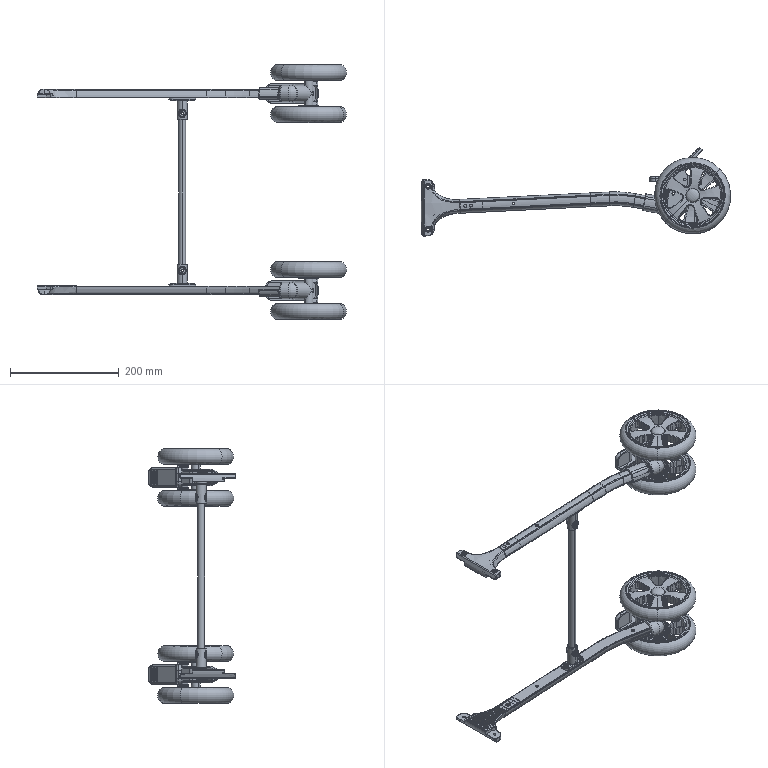Part | SolidWorks | 28 solids | 5292 faces | volume 1062049 mm3 | spline 2261 | cylinder 1472 | plane 1130 | torus 285 | cone 114 | sphere 30 | commonest cylinder face diameters 1 x160 4 x98 3 x81 5.2 x76 2 x74 10 x64